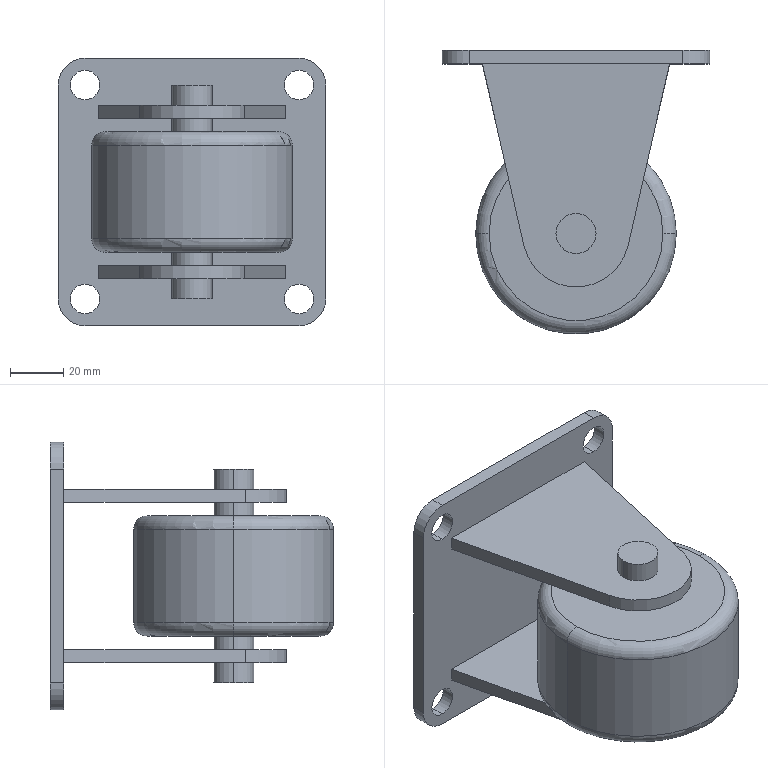Part | STEP file | Caster_default<machined> | 5 solids | 48 faces | box 100 x 106 x 100 mm | volume 289989 mm3 | cylinder 24 | plane 20 | torus 4 | commonest cylinder face diameters 11 x8 15 x8 20 x4 40 x2 75 x2